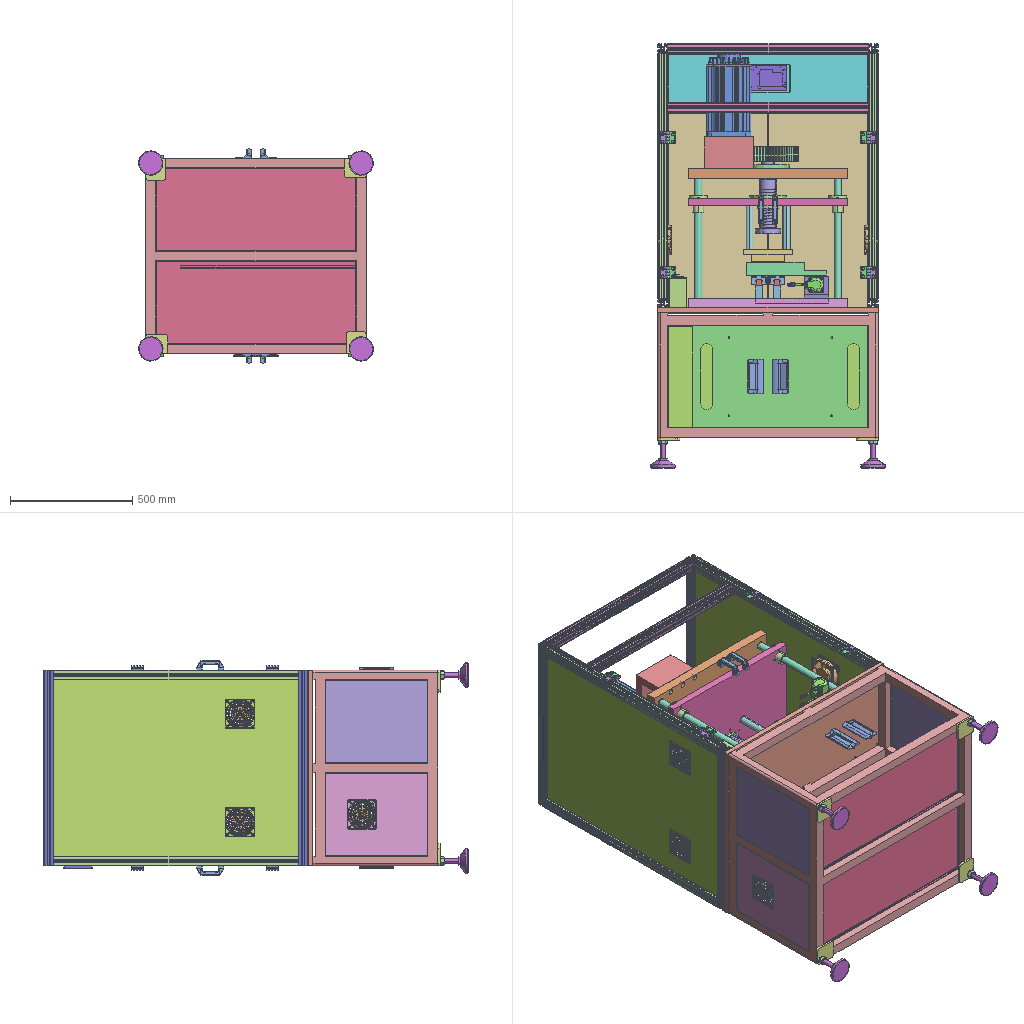Assembly | SolidWorks | 56 different items | 125 placed | box 960 x 1734 x 876 mm
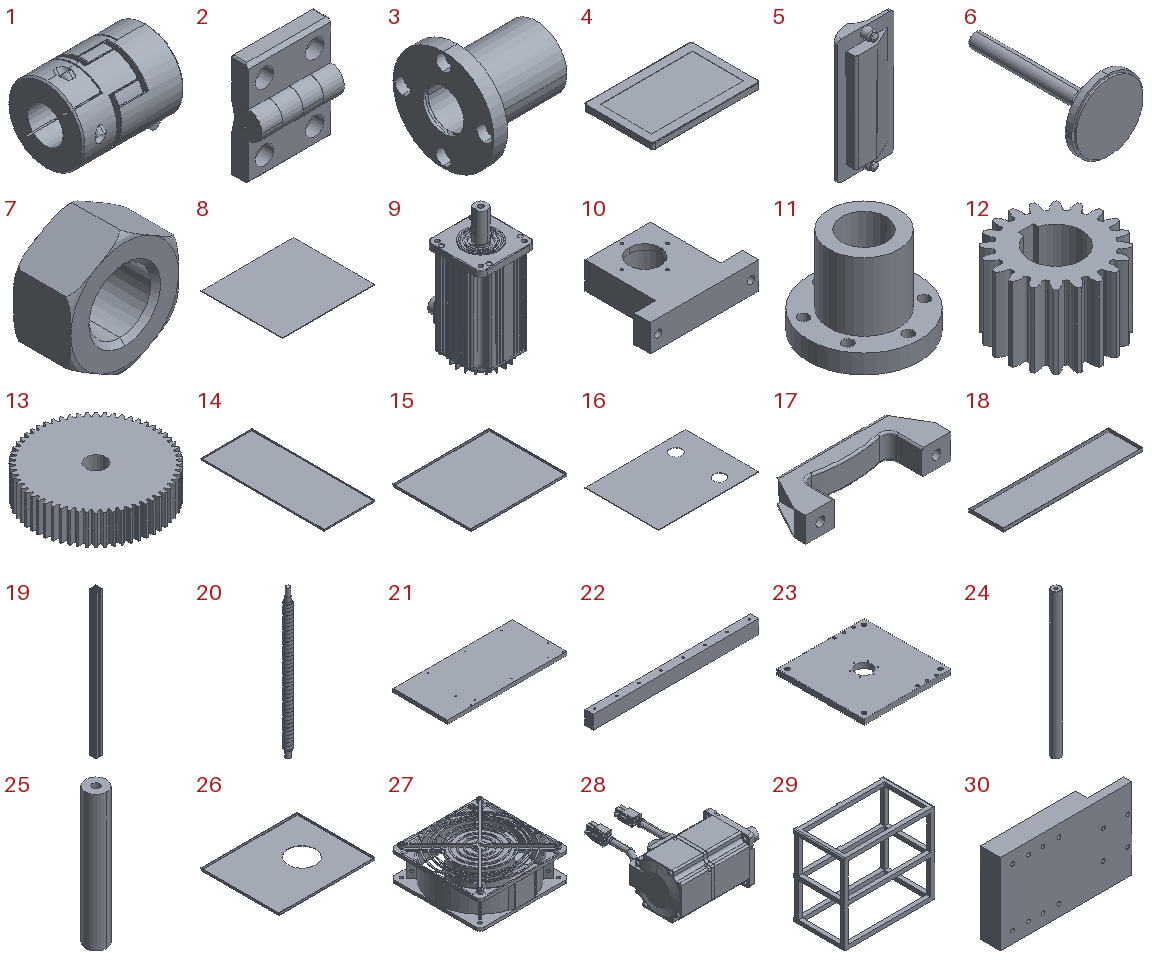Parts list (item | name | quantity | size | volume | features):
1 | - | x1 | 40 x 31.403 x 31.299 mm | 20689 mm3 | features BaseBody 3
2 | - | x8 | 49 x 18 x 62 mm | 30925 mm3 | features BaseBody 3
3 | - | x4 | 68 x 74 x 74 mm | 84248 mm3 | features BaseBody 1
4 | - | x1 | - | - | features RefSurface 1
5 | - | x4 | 64 x 23.592 x 140 mm | 48933 mm3 | features BaseBody 1
6 | - | x4 | 100 x 189 x 100 mm | 224213 mm3 | features BaseBody 1
7 | - | x4 | 30 x 16 x 34.641 mm | 8584 mm3 | features BaseBody 1
8 | - | x1 | 843 x 739 x 5 mm | 3114885 mm3 | features BaseBody 1
9 | - | x1 | 180 x 239.2 x 439.7 mm | 9178277 mm3 | features BaseBody 1
10 | - | x2 | 100 x 80 x 25 mm | 110111 mm3 | features BaseBody 1
11 | - | x1 | 70 x 70 x 55 mm | 72753 mm3 | features BaseBody 1
12 | - | x1 | 87.307 x 87.307 x 60 mm | 210488 mm3 | features BaseBody 1
13 | - | x1 | 247.805 x 247.805 x 60 mm | 2631200 mm3 | features BaseBody 1
14 | - | x2 | 340 x 820 x 10 mm | 590888 mm3 | features BaseBody 1
15 | - | x2 | 420 x 340 x 10 mm | 307281 mm3 | features BaseBody 1
16 | - | x2 | 1023 x 743 x 5 mm | 3687348 mm3 | features BaseBody 1
17 | - | x4 | 110 x 38 x 19 mm | 30744 mm3 | features BaseBody 1
18 | - | x1 | 820 x 200 x 20 mm | 401152 mm3 | features BaseBody 1
19 | - | x4 | 40 x 40 x 820 mm | 575203 mm3 | features BaseBody 1
20 | - | x1 | 28 x 28 x 548 mm | 304343 mm3 | features BaseBody 1
21 | - | x1 | 650 x 300 x 20 mm | 3893705 mm3 | features BaseBody 1
22 | - | x2 | 600 x 30 x 50 mm | 885473 mm3 | features 3DProfileFeature 1, BaseBody 1, HoleWzd 1, LPattern 1
23 | - | x1 | 650 x 650 x 40 mm | 16353197 mm3 | features BaseBody 1
24 | - | x4 | 30 x 30 x 500 mm | 312481 mm3 | features BaseBody 1
25 | - | x4 | 30 x 30 x 190 mm | 118778 mm3 | features BaseBody 1
26 | - | x2 | 420 x 340 x 10 mm | 284661 mm3 | features BaseBody 1
27 | - | x6 | 120 x 120 x 43 mm | 168023 mm3 | features BaseBody 2
28 | - | x1 | 129 x 145.8 x 60 mm | 348980 mm3 | features BaseBody 2
29 | - | x1 | 900 x 510 x 800 mm | 17121482 mm3 | features BaseBody 1
30 | - | x1 | 325 x 50 x 200 mm | 2147505 mm3 | features ICE 3, BaseBody 1
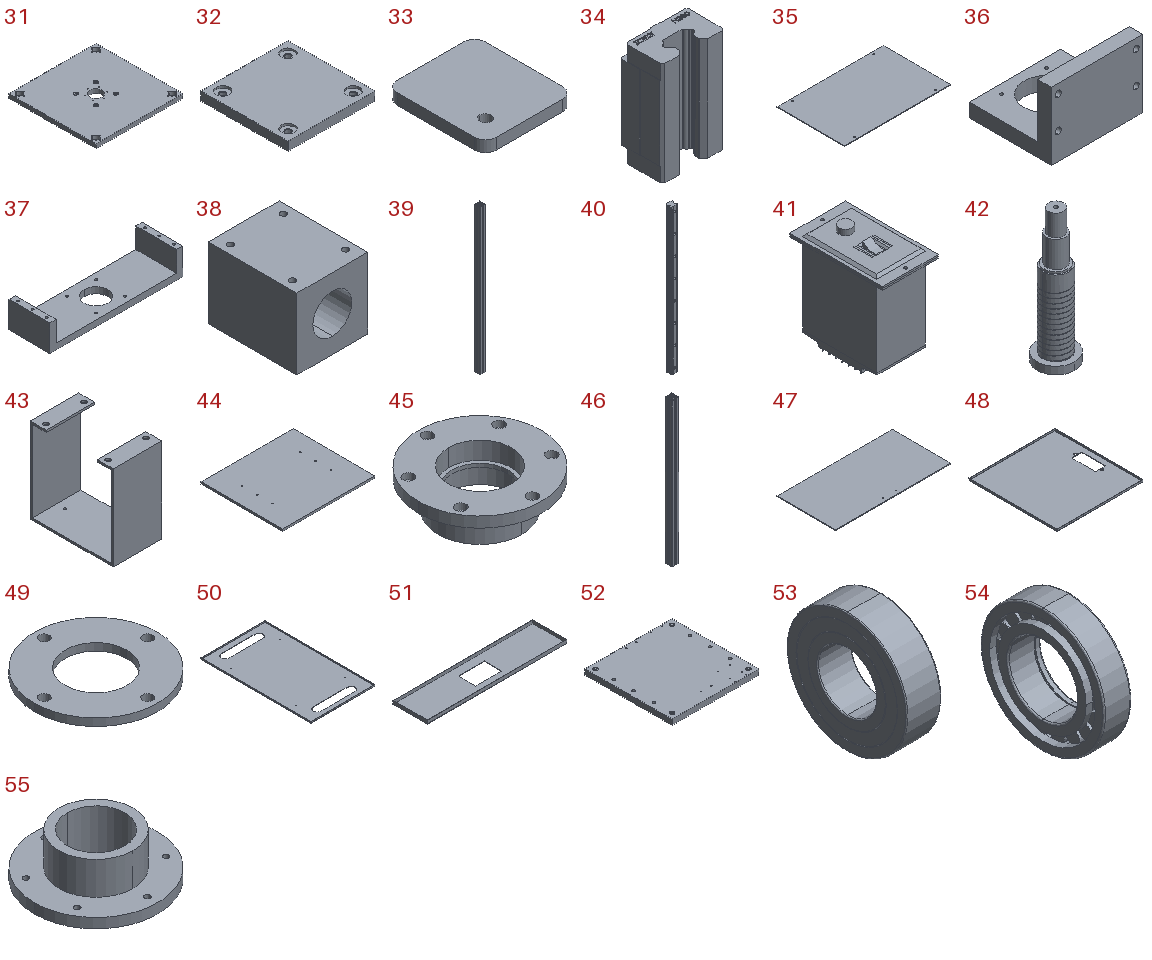31 | - | x1 | 650 x 650 x 30 mm | 12242993 mm3 | features BaseBody 1
32 | - | x1 | 200 x 200 x 50 mm | 1213881 mm3 | features BaseBody 1
33 | - | x4 | 80 x 90 x 10 mm | 70324 mm3 | features BaseBody 1
34 | - | x4 | 60 x 39 x 97.7 mm | 170717 mm3 | features BaseBody 1
35 | - | x1 | 550 x 350 x 3 mm | 577089 mm3 | features BaseBody 1
36 | - | x1 | 100 x 90 x 74 mm | 189827 mm3 | features BaseBody 1
37 | - | x1 | 650 x 200 x 130 mm | 4762030 mm3 | features 3DProfileFeature 1, BaseBody 1, HoleWzd 1, SketchPattern 1
38 | - | x1 | 80 x 100 x 80 mm | 483153 mm3 | features BaseBody 1
39 | - | x4 | 40 x 40 x 1000 mm | 701466 mm3 | features BaseBody 1
40 | - | x2 | 28 x 26 x 600 mm | 346046 mm3 | features BaseBody 1
41 | - | x2 | 60 x 100 x 107 mm | 402424 mm3 | features BaseBody 3
42 | - | x1 | 100 x 100 x 352 mm | 1147251 mm3 | features BaseBody 1
43 | - | x2 | 70 x 120 x 123 mm | 83550 mm3 | features 3DProfileFeature 1, BaseBody 1, HoleWzd 1
44 | - | x1 | 900 x 800 x 20 mm | 14390194 mm3 | features BaseBody 1
45 | - | x1 | 176 x 176 x 55 mm | 462265 mm3 | features BaseBody 1
46 | - | x4 | 40 x 40 x 800 mm | 561173 mm3 | features BaseBody 1
47 | - | x4 | 796 x 405 x 5 mm | 1611704 mm3 | features BaseBody 1
48 | - | x4 | 410 x 420 x 10 mm | 356908 mm3 | features BaseBody 1
49 | - | x3 | 50 x 50 x 3 mm | 4267 mm3 | features BaseBody 1
50 | - | x1 | 420 x 720 x 25 mm | 587350 mm3 | features BaseBody 1
51 | - | x1 | 820 x 200 x 20 mm | 369634 mm3 | features BaseBody 1
52 | - | x1 | 650 x 650 x 40 mm | 16789286 mm3 | features BaseBody 1
53 | - | x4 | 10 x 35 x 35 mm | 5537 mm3 | features BaseBody 17
54 | - | x2 | 24 x 90 x 90 mm | 70515 mm3 | features BaseBody 20
55 | - | x1 | 150 x 150 x 52 mm | 261462 mm3 | features BaseBody 1
56 | Washer | x1 | - | - | -